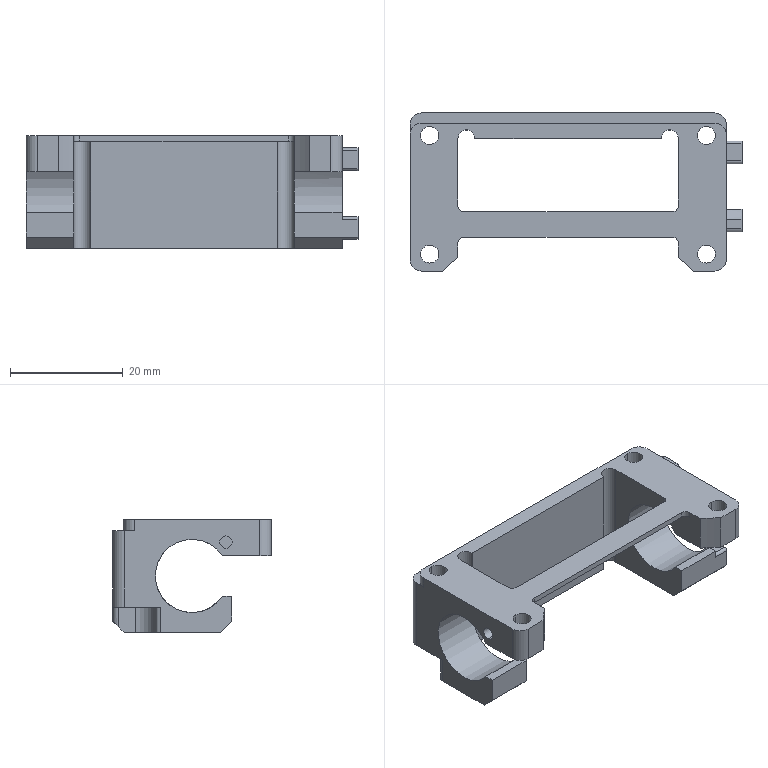CAM job | Mastercam | 3-axis milling, 5-axis milling, drilling | part box 58.8 x 28 x 20 mm | stock box 69 x 38 x 20 mm
Tools:
tool_number,name,type,diameter_mm,corner_radius_mm,flutes,flute_length_mm,overall_length_mm,shoulder_length_mm,holder_diameter_mm,length_offset,diameter_offset,default_rpm,default_feed_mm_min,default_plunge_mm_min,coolant
1,3 Drill,drill,3,0,2,25,50,40,50,1,1,1200,100,600,COOL_OFF
2,2 Flat End Mill,end mill,2,0,4,25,75,25,50,2,2,6500,2000,600,COOL_OFF
3,3 Flat End Mill,end mill,3,0,4,25,75,25,50,3,3,6000,2000,600,COOL_OFF
5,4 Chamfer Mill,chamfer mill,4,0,4,25,75,30,50,5,5,6250,750,600,COOL_OFF
6,6 Flat End Mill,end mill,6,0,4,25,75,25,50,6,6,6500,2500,600,COOL_OFF
7,4 Chamfer Mill,chamfer mill,4,0,4,25,75,30,50,7,7,3000,300,600,COOL_OFF
8,8 Flat End Mill,end mill,8,0,4,25,75,25,50,8,8,6000,3000,600,COOL_OFF
9,10 Flat End Mill,end mill,10,0,4,25,75,25,50,9,9,1000,120,600,COOL_OFF
10,10 Flat End Mill,end mill,10,0,4,25,75,25,50,10,10,6500,4000,600,COOL_OFF
18,8 Bull Nose Mill,bull end mill,8,1,4,25,100,25,50,18,18,7000,3000,600,COOL_OFF
24,100 Flat End Mill,end mill,100,0,4,25,75,25,50,24,24,4000,1000,600,COOL_OFF
Operations:
seq,operation,operation_type,tool_number,tool_name,tool_diameter_mm,spindle_rpm,feed_mm_min,plunge_mm_min,retract_mm_min,cycle_time_s,wcs,posted,nc_file
1,Facing - [WCS: Plane] - [Tplane: Plane],Facing,24,100 Flat End Mill,100,4000,1000,600,1200,14.075,Plane,yes,.nc
2,Drill/Counterbore - [WCS: Plane] - [Tplane: Plane],Drill,7,4 Chamfer Mill,4,3000,300,600,1200,1.637,Plane,yes,.nc
3,Peck Drill - [WCS: Plane] - [Tplane: Plane],Drill,1,3 Drill,3,1200,100,600,1200,32.506,Plane,yes,.nc
4,Surface Rough Pocket - [WCS: Plane] - [Tplane: Plane],MultiSurfaceRoughPocket,10,10 Flat End Mill,10,6500,4000,600,1200,385.383,Plane,yes,.nc
5,3D High Speed (Waterline rest passes) - [WCS: Plane] - [Tplane: Plane],HighSpeed3D,6,6 Flat End Mill,6,6500,2500,600,1200,78.996,Plane,yes,.nc
6,Contour (Remachining) - [WCS: Plane] - [Tplane: Plane],Contour,3,3 Flat End Mill,3,6000,2000,600,1200,42.799,Plane,yes,.nc
7,Contour (2D) - [WCS: Plane] - [Tplane: Plane],Contour,6,6 Flat End Mill,6,6500,1000,600,1200,22.816,Plane,yes,.nc
8,Contour (2D) - [WCS: Plane] - [Tplane: Plane],Contour,6,6 Flat End Mill,6,6500,1000,600,1200,8.739,Plane,yes,.nc
9,Contour (2D) - [WCS: Plane] - [Tplane: Plane],Contour,6,6 Flat End Mill,6,6500,1000,600,1200,5.555,Plane,yes,.nc
10,Contour (2D) - [WCS: Plane] - [Tplane: Plane],Contour,6,6 Flat End Mill,6,6500,1000,600,1200,7.096,Plane,yes,.nc
11,Contour (2D) - [WCS: Plane] - [Tplane: Plane],Contour,6,6 Flat End Mill,6,6500,1000,600,1200,5.762,Plane,yes,.nc
12,Contour (2D) - [WCS: Plane] - [Tplane: Plane],Contour,6,6 Flat End Mill,6,6500,1000,600,1200,8.286,Plane,yes,.nc
13,Contour (2D) - [WCS: Plane] - [Tplane: Plane],Contour,6,6 Flat End Mill,6,6500,1000,600,1200,27.364,Plane,yes,.nc
14,Surface Finish Parallel - [WCS: Plane] - [Tplane: Plane],MultiSurfaceFinishParallel,18,8 Bull Nose Mill,8,7000,3000,600,1200,37.534,Plane,yes,.nc
15,Deburr 5-axis - [WCS: Plane] - [Tplane: Plane],459,7,4 Chamfer Mill,4,6500,1000,600,1200,21.825,Plane,yes,.nc
16,Drill/Counterbore - [WCS: Plane] - [Tplane: Plane],Drill,7,4 Chamfer Mill,4,3000,300,600,1200,3.622,Plane,yes,.nc
17,Contour (2D) - [WCS: Plane-1] - [Tplane: Plane-1],Contour,10,10 Flat End Mill,10,6500,3000,600,1200,51.153,Plane-1,yes,.nc
18,Facing - [WCS: Plane-1] - [Tplane: Plane-1],Facing,24,100 Flat End Mill,100,4000,3000,600,1200,99.629,Plane-1,yes,.nc
19,Facing - [WCS: Plane-1] - [Tplane: Plane-1],Facing,6,6 Flat End Mill,6,6500,1000,600,1200,44.437,Plane-1,yes,.nc
20,Contour (Ramp) - [WCS: Plane-1] - [Tplane: Plane-1],Contour,6,6 Flat End Mill,6,6500,4000,600,1200,4.801,Plane-1,yes,.nc
21,Contour (2D) - [WCS: Plane-1] - [Tplane: Plane-1],Contour,6,6 Flat End Mill,6,6500,1000,600,1200,4.792,Plane-1,yes,.nc
22,Contour (Remachining) - [WCS: Plane-1] - [Tplane: Plane-1],Contour,2,2 Flat End Mill,2,6500,1500,600,1200,3.465,Plane-1,yes,.nc
23,Contour (2D chamfer) - [WCS: Plane-1] - [Tplane: Plane-1],Contour,7,4 Chamfer Mill,4,6500,1000,600,1200,6.658,Plane-1,yes,.nc
24,Contour (2D chamfer) - [WCS: Plane-1] - [Tplane: Plane-1],Contour,7,4 Chamfer Mill,4,6500,1000,600,1200,9.655,Plane-1,yes,.nc
25,Contour (Ramp) - [WCS: Plane-2] - [Tplane: Plane-2],Contour,6,6 Flat End Mill,6,6000,3000,600,1200,6.103,Plane-2,yes,.nc
26,Contour (2D) - [WCS: Plane-2] - [Tplane: Plane-2],Contour,6,6 Flat End Mill,6,6000,3000,600,1200,16.066,Plane-2,yes,.nc
27,Contour (2D) - [WCS: Plane-2] - [Tplane: Plane-2],Contour,6,6 Flat End Mill,6,6000,1000,600,1200,6.49,Plane-2,yes,.nc
28,Contour (2D) - [WCS: Plane-2] - [Tplane: Plane-2],Contour,6,6 Flat End Mill,6,6500,1000,600,1200,2.221,Plane-2,yes,.nc
29,Contour (2D chamfer) - [WCS: Plane-2] - [Tplane: Plane-2],Contour,5,4 Chamfer Mill,4,7000,1000,600,1200,3.775,Plane-2,yes,.nc
30,Drill/Counterbore - [WCS: Plane-2] - [Tplane: Plane-2],Drill,5,4 Chamfer Mill,4,3000,300,600,1200,0.819,Plane-2,yes,.nc
31,3D High Speed (Horizontal) - [WCS: Plane-3] - [Tplane: Plane-3],HighSpeed3D,6,6 Flat End Mill,6,6500,3000,600,1200,43.246,Plane-3,yes,.nc
32,Contour (Ramp) - [WCS: Plane-3] - [Tplane: Plane-3],Contour,6,6 Flat End Mill,6,6500,3000,600,1200,9.586,Plane-3,yes,.nc
33,3D High Speed (Horizontal) - [WCS: Plane-3] - [Tplane: Plane-3],HighSpeed3D,6,6 Flat End Mill,6,6500,1000,600,1200,20.079,Plane-3,yes,.nc
34,Contour (2D) - [WCS: Plane-3] - [Tplane: Plane-3],Contour,6,6 Flat End Mill,6,6500,1000,600,1200,5.069,Plane-3,yes,.nc
35,Contour (Ramp) - [WCS: Plane-3] - [Tplane: Plane-3],Contour,6,6 Flat End Mill,6,6500,3000,600,1200,3.922,Plane-3,yes,.nc
36,Contour (2D) - [WCS: Plane-3] - [Tplane: Plane-3],Contour,6,6 Flat End Mill,6,6500,3000,600,1200,16.862,Plane-3,yes,.nc
37,Contour (2D) - [WCS: Plane-3] - [Tplane: Plane-3],Contour,6,6 Flat End Mill,6,6500,1000,600,1200,6.496,Plane-3,yes,.nc
38,Contour (2D) - [WCS: Plane-3] - [Tplane: Plane-3],Contour,6,6 Flat End Mill,6,6500,1000,600,1200,2.416,Plane-3,yes,.nc
39,Drill/Counterbore - [WCS: Plane-3] - [Tplane: Plane-3],Drill,5,4 Chamfer Mill,4,3000,300,600,1200,2.483,Plane-3,yes,.nc
40,Deburr 5-axis - [WCS: Plane-3] - [Tplane: Plane-3],459,5,4 Chamfer Mill,4,6500,1000,600,1200,10.698,Plane-3,yes,.nc
41,Surface Finish Flowline - [WCS: Plane-3] - [Tplane: Plane-3],MultiSurfaceFinishFlowline,18,8 Bull Nose Mill,8,7000,3000,600,1200,27.043,Plane-3,yes,.nc
42,Contour (Ramp) - [WCS: Plane-4] - [Tplane: Plane-4],Contour,6,6 Flat End Mill,6,6500,1000,600,1200,97.536,Plane-4,yes,.nc
43,Contour (2D) - [WCS: Plane-4] - [Tplane: Plane-4],Contour,6,6 Flat End Mill,6,6500,1000,600,1200,3.945,Plane-4,yes,.nc
44,Facing - [WCS: Plane-5] - [Tplane: Plane-5],Facing,24,100 Flat End Mill,100,4000,3000,600,1200,52.895,Plane-5,yes,.nc
45,Contour (Ramp) - [WCS: Plane-5] - [Tplane: Plane-5],Contour,9,10 Flat End Mill,10,6500,4000,600,1200,94.896,Plane-5,yes,.nc
46,Contour (2D) - [WCS: Plane-5] - [Tplane: Plane-5],Contour,10,10 Flat End Mill,10,6500,1000,600,1200,12.129,Plane-5,yes,.nc
47,Contour (2D chamfer) - [WCS: Plane-5] - [Tplane: Plane-5],Contour,7,4 Chamfer Mill,4,6500,1000,600,1200,8.323,Plane-5,yes,.nc